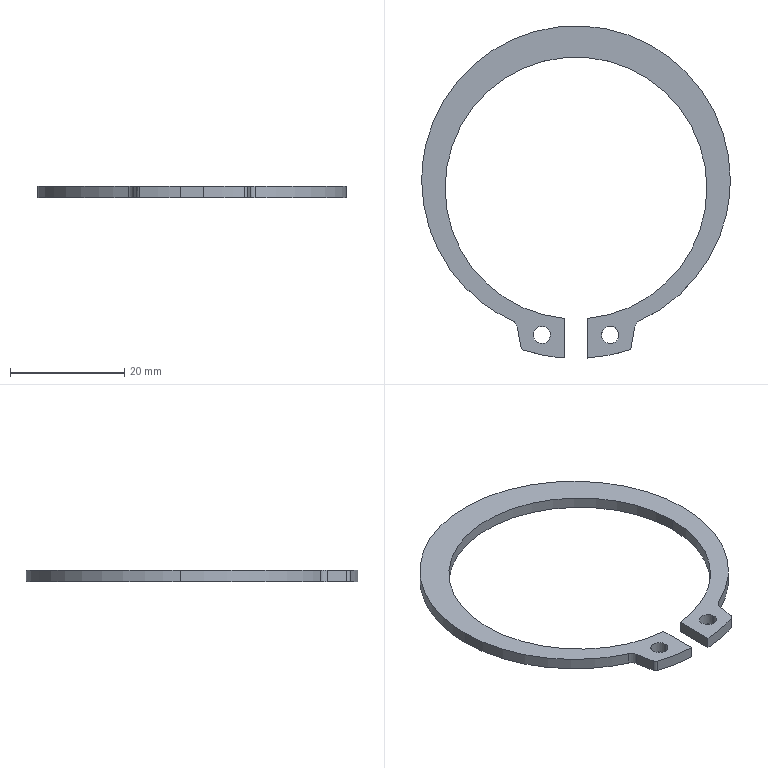Part | STEP file | PN_0041_Default<As Machined> | 1 solid | 22 faces | box 54 x 58.103 x 2 mm | volume 1371 mm3 | cylinder 16 | plane 6 | commonest cylinder face diameters 3 x6 45.8 x3 54 x3 1.4 x2 59.6 x2
STEP:
#1=CARTESIAN_POINT('',(4.5,-27.079,-2.));
#2=VERTEX_POINT('',#1);
#3=CARTESIAN_POINT('',(7.5,-27.079,-2.));
#4=VERTEX_POINT('',#3);
#5=CARTESIAN_POINT('',(6.,-27.079,-2.));
#6=DIRECTION('',(0.,0.,1.));
#7=AXIS2_PLACEMENT_3D('',#5,#6,$);
#8=CIRCLE('',#7,1.5);
#9=EDGE_CURVE('',#2,#4,#8,.T.);
#10=ORIENTED_EDGE('',*,*,#9,.F.);
#11=CARTESIAN_POINT('',(4.5,-27.079,0.));
#12=VERTEX_POINT('',#11);
#13=CARTESIAN_POINT('',(4.5,-27.079,-2.));
#14=DIRECTION('',(0.,0.,1.));
#15=VECTOR('',#14,1.);
#16=LINE('',#13,#15);
#17=EDGE_CURVE('',#2,#12,#16,.T.);
#18=ORIENTED_EDGE('',*,*,#17,.T.);
#19=CARTESIAN_POINT('',(7.5,-27.079,0.));
#20=VERTEX_POINT('',#19);
#21=CARTESIAN_POINT('',(6.,-27.079,0.));
#22=DIRECTION('',(0.,0.,1.));
#23=AXIS2_PLACEMENT_3D('',#21,#22,$);
#24=CIRCLE('',#23,1.5);
#25=EDGE_CURVE('',#12,#20,#24,.T.);
#26=ORIENTED_EDGE('',*,*,#25,.T.);
#27=CARTESIAN_POINT('',(7.5,-27.079,-2.));
#28=DIRECTION('',(0.,0.,1.));
#29=VECTOR('',#28,1.);
#30=LINE('',#27,#29);
#31=EDGE_CURVE('',#4,#20,#30,.T.);
#32=ORIENTED_EDGE('',*,*,#31,.F.);
#33=EDGE_LOOP('',(#10,#18,#26,#32));
#34=FACE_OUTER_BOUND('',#33,.T.);
#35=CARTESIAN_POINT('',(6.,-27.079,-2.));
#36=DIRECTION('',(0.,0.,1.));
#37=DIRECTION('',(-1.,0.,0.));
#38=AXIS2_PLACEMENT_3D('',#35,#36,#37);
#39=CYLINDRICAL_SURFACE('',#38,1.5);
#40=ADVANCED_FACE('',(#34),#39,.F.);
#41=CARTESIAN_POINT('',(-9.187,-29.719,-2.));
#42=VERTEX_POINT('',#41);
#43=CARTESIAN_POINT('',(-2.,-31.103,-2.));
#44=VERTEX_POINT('',#43);
#45=CARTESIAN_POINT('',(-9.187,-29.719,-2.));
#46=CARTESIAN_POINT('',(-7.791,-30.171,-2.));
#47=CARTESIAN_POINT('',(-6.367,-30.537,-2.));
#48=CARTESIAN_POINT('',(-4.922,-30.816,-2.));
#49=CARTESIAN_POINT('',(-3.464,-31.004,-2.));
#50=CARTESIAN_POINT('',(-2.,-31.103,-2.));
#51=B_SPLINE_CURVE_WITH_KNOTS('',5,(#45,#46,#47,#48,#49,#50),.UNSPECIFIED.,.F.,.U.,(6,6),(0.,10.377),.UNSPECIFIED.);
#52=EDGE_CURVE('',#42,#44,#51,.T.);
#53=ORIENTED_EDGE('',*,*,#52,.F.);
#54=CARTESIAN_POINT('',(-9.66,-29.174,-2.));
#55=VERTEX_POINT('',#54);
#56=CARTESIAN_POINT('',(-8.971,-29.053,-2.));
#57=DIRECTION('',(0.,0.,-1.));
#58=AXIS2_PLACEMENT_3D('',#56,#57,$);
#59=CIRCLE('',#58,0.7);
#60=EDGE_CURVE('',#42,#55,#59,.T.);
#61=ORIENTED_EDGE('',*,*,#60,.T.);
#62=CARTESIAN_POINT('',(-10.272,-25.705,-2.));
#63=VERTEX_POINT('',#62);
#64=CARTESIAN_POINT('',(-9.966,-27.44,-2.));
#65=DIRECTION('',(0.1736,-0.9848,0.));
#66=VECTOR('',#65,1.);
#67=LINE('',#64,#66);
#68=EDGE_CURVE('',#63,#55,#67,.T.);
#69=ORIENTED_EDGE('',*,*,#68,.F.);
#70=CARTESIAN_POINT('',(-11.131,-24.599,-2.));
#71=VERTEX_POINT('',#70);
#72=CARTESIAN_POINT('',(-10.272,-25.705,-2.));
#73=CARTESIAN_POINT('',(-10.303,-25.533,-2.));
#74=CARTESIAN_POINT('',(-10.358,-25.365,-2.));
#75=CARTESIAN_POINT('',(-10.438,-25.207,-2.));
#76=CARTESIAN_POINT('',(-10.607,-24.966,-2.));
#77=CARTESIAN_POINT('',(-10.828,-24.773,-2.));
#78=CARTESIAN_POINT('',(-10.923,-24.705,-2.));
#79=CARTESIAN_POINT('',(-11.025,-24.647,-2.));
#80=CARTESIAN_POINT('',(-11.131,-24.599,-2.));
#81=B_SPLINE_CURVE_WITH_KNOTS('',5,(#72,#73,#74,#75,#76,#77,#78,#79,#80),.UNSPECIFIED.,.F.,.U.,(6,3,6),(0.,1.236,2.06),.UNSPECIFIED.);
#82=EDGE_CURVE('',#63,#71,#81,.T.);
#83=ORIENTED_EDGE('',*,*,#82,.T.);
#84=CARTESIAN_POINT('',(-27.,0.,-2.));
#85=VERTEX_POINT('',#84);
#86=CARTESIAN_POINT('',(-27.,-0.000000001,-2.));
#87=CARTESIAN_POINT('',(-27.,-2.546,-2.));
#88=CARTESIAN_POINT('',(-26.7,-5.091,-2.));
#89=CARTESIAN_POINT('',(-26.1,-7.59,-2.));
#90=CARTESIAN_POINT('',(-24.322,-12.398,-2.));
#91=CARTESIAN_POINT('',(-21.476,-16.661,-2.));
#92=CARTESIAN_POINT('',(-19.807,-18.615,-2.));
#93=CARTESIAN_POINT('',(-17.111,-21.102,-2.));
#94=CARTESIAN_POINT('',(-14.056,-23.092,-2.));
#95=CARTESIAN_POINT('',(-13.106,-23.644,-2.));
#96=CARTESIAN_POINT('',(-12.13,-24.147,-2.));
#97=CARTESIAN_POINT('',(-11.131,-24.599,-2.));
#98=B_SPLINE_CURVE_WITH_KNOTS('',5,(#86,#87,#88,#89,#90,#91,#92,#93,#94,#95,#96,#97),.UNSPECIFIED.,.F.,.U.,(6,3,3,6),(0.,18.,36.,43.753),.UNSPECIFIED.);
#99=EDGE_CURVE('',#85,#71,#98,.T.);
#100=ORIENTED_EDGE('',*,*,#99,.F.);
#101=CARTESIAN_POINT('',(27.,0.,-2.));
#102=VERTEX_POINT('',#101);
#103=CARTESIAN_POINT('',(27.,-0.000000001,-2.));
#104=CARTESIAN_POINT('',(27.,2.546,-2.));
#105=CARTESIAN_POINT('',(26.7,5.091,-2.));
#106=CARTESIAN_POINT('',(26.1,7.59,-2.));
#107=CARTESIAN_POINT('',(24.322,12.398,-2.));
#108=CARTESIAN_POINT('',(21.476,16.661,-2.));
#109=CARTESIAN_POINT('',(19.807,18.615,-2.));
#110=CARTESIAN_POINT('',(16.039,22.091,-2.));
#111=CARTESIAN_POINT('',(11.567,24.597,-2.));
#112=CARTESIAN_POINT('',(9.193,25.579,-2.));
#113=CARTESIAN_POINT('',(4.257,26.966,-2.));
#114=CARTESIAN_POINT('',(-0.8651,27.167,-2.));
#115=CARTESIAN_POINT('',(-3.427,26.964,-2.));
#116=CARTESIAN_POINT('',(-8.453,25.958,-2.));
#117=CARTESIAN_POINT('',(-13.108,23.811,-2.));
#118=CARTESIAN_POINT('',(-15.298,22.467,-2.));
#119=CARTESIAN_POINT('',(-19.32,19.288,-2.));
#120=CARTESIAN_POINT('',(-22.492,15.261,-2.));
#121=CARTESIAN_POINT('',(-23.833,13.069,-2.));
#122=CARTESIAN_POINT('',(-25.613,9.192,-2.));
#123=CARTESIAN_POINT('',(-26.603,5.059,-2.));
#124=CARTESIAN_POINT('',(-26.868,3.382,-2.));
#125=CARTESIAN_POINT('',(-27.,1.691,-2.));
#126=CARTESIAN_POINT('',(-27.,-0.000000001,-2.));
#127=B_SPLINE_CURVE_WITH_KNOTS('',5,(#103,#104,#105,#106,#107,#108,#109,#110,#111,#112,#113,#114,#115,#116,#117,#118,#119,#120,#121,#122,#123,#124,#125,#126),.UNSPECIFIED.,.F.,.U.,(6,3,3,3,3,3,3,6),(0.,18.,36.,54.,71.999,89.999,107.999,119.957),.UNSPECIFIED.);
#128=EDGE_CURVE('',#102,#85,#127,.T.);
#129=ORIENTED_EDGE('',*,*,#128,.F.);
#130=CARTESIAN_POINT('',(11.131,-24.599,-2.));
#131=VERTEX_POINT('',#130);
#132=CARTESIAN_POINT('',(11.131,-24.599,-2.));
#133=CARTESIAN_POINT('',(13.45,-23.549,-2.));
#134=CARTESIAN_POINT('',(15.646,-22.227,-2.));
#135=CARTESIAN_POINT('',(17.675,-20.65,-2.));
#136=CARTESIAN_POINT('',(21.323,-17.048,-2.));
#137=CARTESIAN_POINT('',(24.033,-12.697,-2.));
#138=CARTESIAN_POINT('',(25.125,-10.371,-2.));
#139=CARTESIAN_POINT('',(26.28,-6.89,-2.));
#140=CARTESIAN_POINT('',(26.833,-3.286,-2.));
#141=CARTESIAN_POINT('',(26.944,-2.193,-2.));
#142=CARTESIAN_POINT('',(27.,-1.096,-2.));
#143=CARTESIAN_POINT('',(27.,-0.000000001,-2.));
#144=B_SPLINE_CURVE_WITH_KNOTS('',5,(#132,#133,#134,#135,#136,#137,#138,#139,#140,#141,#142,#143),.UNSPECIFIED.,.F.,.U.,(6,3,3,6),(0.,18.,36.,43.753),.UNSPECIFIED.);
#145=EDGE_CURVE('',#131,#102,#144,.T.);
#146=ORIENTED_EDGE('',*,*,#145,.F.);
#147=CARTESIAN_POINT('',(10.272,-25.705,-2.));
#148=VERTEX_POINT('',#147);
#149=CARTESIAN_POINT('',(11.131,-24.599,-2.));
#150=CARTESIAN_POINT('',(10.972,-24.671,-2.));
#151=CARTESIAN_POINT('',(10.823,-24.766,-2.));
#152=CARTESIAN_POINT('',(10.689,-24.883,-2.));
#153=CARTESIAN_POINT('',(10.498,-25.106,-2.));
#154=CARTESIAN_POINT('',(10.366,-25.368,-2.));
#155=CARTESIAN_POINT('',(10.324,-25.477,-2.));
#156=CARTESIAN_POINT('',(10.292,-25.59,-2.));
#157=CARTESIAN_POINT('',(10.272,-25.705,-2.));
#158=B_SPLINE_CURVE_WITH_KNOTS('',5,(#149,#150,#151,#152,#153,#154,#155,#156,#157),.UNSPECIFIED.,.F.,.U.,(6,3,6),(0.,1.236,2.06),.UNSPECIFIED.);
#159=EDGE_CURVE('',#131,#148,#158,.T.);
#160=ORIENTED_EDGE('',*,*,#159,.T.);
#161=CARTESIAN_POINT('',(9.66,-29.174,-2.));
#162=VERTEX_POINT('',#161);
#163=CARTESIAN_POINT('',(9.966,-27.44,-2.));
#164=DIRECTION('',(0.1736,0.9848,0.));
#165=VECTOR('',#164,1.);
#166=LINE('',#163,#165);
#167=EDGE_CURVE('',#162,#148,#166,.T.);
#168=ORIENTED_EDGE('',*,*,#167,.F.);
#169=CARTESIAN_POINT('',(9.187,-29.719,-2.));
#170=VERTEX_POINT('',#169);
#171=CARTESIAN_POINT('',(8.971,-29.053,-2.));
#172=DIRECTION('',(0.,0.,-1.));
#173=AXIS2_PLACEMENT_3D('',#171,#172,$);
#174=CIRCLE('',#173,0.7);
#175=EDGE_CURVE('',#162,#170,#174,.T.);
#176=ORIENTED_EDGE('',*,*,#175,.T.);
#177=CARTESIAN_POINT('',(2.,-31.103,-2.));
#178=VERTEX_POINT('',#177);
#179=CARTESIAN_POINT('',(2.,-31.103,-2.));
#180=CARTESIAN_POINT('',(3.464,-31.004,-2.));
#181=CARTESIAN_POINT('',(4.922,-30.816,-2.));
#182=CARTESIAN_POINT('',(6.367,-30.537,-2.));
#183=CARTESIAN_POINT('',(7.791,-30.171,-2.));
#184=CARTESIAN_POINT('',(9.187,-29.719,-2.));
#185=B_SPLINE_CURVE_WITH_KNOTS('',5,(#179,#180,#181,#182,#183,#184),.UNSPECIFIED.,.F.,.U.,(6,6),(0.,10.377),.UNSPECIFIED.);
#186=EDGE_CURVE('',#178,#170,#185,.T.);
#187=ORIENTED_EDGE('',*,*,#186,.F.);
#188=CARTESIAN_POINT('',(2.,-24.182,-2.));
#189=VERTEX_POINT('',#188);
#190=CARTESIAN_POINT('',(2.,-27.643,-2.));
#191=DIRECTION('',(0.,-1.,0.));
#192=VECTOR('',#191,1.);
#193=LINE('',#190,#192);
#194=EDGE_CURVE('',#189,#178,#193,.T.);
#195=ORIENTED_EDGE('',*,*,#194,.F.);
#196=CARTESIAN_POINT('',(22.9,-1.37,-2.));
#197=VERTEX_POINT('',#196);
#198=CARTESIAN_POINT('',(0.000000001,-1.37,-2.));
#199=DIRECTION('',(0.,0.,-1.));
#200=AXIS2_PLACEMENT_3D('',#198,#199,$);
#201=CIRCLE('',#200,22.9);
#202=EDGE_CURVE('',#197,#189,#201,.T.);
#203=ORIENTED_EDGE('',*,*,#202,.F.);
#204=CARTESIAN_POINT('',(-22.9,-1.37,-2.));
#205=VERTEX_POINT('',#204);
#206=CARTESIAN_POINT('',(0.,-1.37,-2.));
#207=DIRECTION('',(0.,0.,-1.));
#208=AXIS2_PLACEMENT_3D('',#206,#207,$);
#209=CIRCLE('',#208,22.9);
#210=EDGE_CURVE('',#205,#197,#209,.T.);
#211=ORIENTED_EDGE('',*,*,#210,.F.);
#212=CARTESIAN_POINT('',(-2.,-24.182,-2.));
#213=VERTEX_POINT('',#212);
#214=CARTESIAN_POINT('',(-0.000000001,-1.37,-2.));
#215=DIRECTION('',(0.,0.,-1.));
#216=AXIS2_PLACEMENT_3D('',#214,#215,$);
#217=CIRCLE('',#216,22.9);
#218=EDGE_CURVE('',#213,#205,#217,.T.);
#219=ORIENTED_EDGE('',*,*,#218,.F.);
#220=CARTESIAN_POINT('',(-2.,-27.643,-2.));
#221=DIRECTION('',(0.,1.,0.));
#222=VECTOR('',#221,1.);
#223=LINE('',#220,#222);
#224=EDGE_CURVE('',#44,#213,#223,.T.);
#225=ORIENTED_EDGE('',*,*,#224,.F.);
#226=EDGE_LOOP('',(#53,#61,#69,#83,#100,#129,#146,#160,#168,#176,#187,#195,#203,#211,#219,#225));
#227=FACE_OUTER_BOUND('',#226,.T.);
#228=CARTESIAN_POINT('',(7.5,-27.079,-2.));
#229=CARTESIAN_POINT('',(7.5,-26.899,-2.));
#230=CARTESIAN_POINT('',(7.473,-26.719,-2.));
#231=CARTESIAN_POINT('',(7.419,-26.545,-2.));
#232=CARTESIAN_POINT('',(7.26,-26.217,-2.));
#233=CARTESIAN_POINT('',(7.012,-25.95,-2.));
#234=CARTESIAN_POINT('',(6.869,-25.837,-2.));
#235=CARTESIAN_POINT('',(6.553,-25.656,-2.));
#236=CARTESIAN_POINT('',(6.198,-25.576,-2.));
#237=CARTESIAN_POINT('',(6.016,-25.563,-2.));
#238=CARTESIAN_POINT('',(5.653,-25.592,-2.));
#239=CARTESIAN_POINT('',(5.315,-25.726,-2.));
#240=CARTESIAN_POINT('',(5.157,-25.819,-2.));
#241=CARTESIAN_POINT('',(4.874,-26.048,-2.));
#242=CARTESIAN_POINT('',(4.671,-26.35,-2.));
#243=CARTESIAN_POINT('',(4.593,-26.515,-2.));
#244=CARTESIAN_POINT('',(4.528,-26.73,-2.));
#245=CARTESIAN_POINT('',(4.505,-26.952,-2.));
#246=CARTESIAN_POINT('',(4.502,-26.994,-2.));
#247=CARTESIAN_POINT('',(4.5,-27.037,-2.));
#248=CARTESIAN_POINT('',(4.5,-27.079,-2.));
#249=B_SPLINE_CURVE_WITH_KNOTS('',5,(#228,#229,#230,#231,#232,#233,#234,#235,#236,#237,#238,#239,#240,#241,#242,#243,#244,#245,#246,#247,#248),.UNSPECIFIED.,.F.,.U.,(6,3,3,3,3,3,6),(0.,1.273,2.546,3.818,5.091,6.364,6.664),.UNSPECIFIED.);
#250=EDGE_CURVE('',#4,#2,#249,.T.);
#251=ORIENTED_EDGE('',*,*,#250,.T.);
#252=ORIENTED_EDGE('',*,*,#9,.T.);
#253=EDGE_LOOP('',(#251,#252));
#254=FACE_BOUND('',#253,.T.);
#255=CARTESIAN_POINT('',(-4.5,-27.079,-2.));
#256=VERTEX_POINT('',#255);
#257=CARTESIAN_POINT('',(-7.5,-27.079,-2.));
#258=VERTEX_POINT('',#257);
#259=CARTESIAN_POINT('',(-4.5,-27.079,-2.));
#260=CARTESIAN_POINT('',(-4.5,-26.899,-2.));
#261=CARTESIAN_POINT('',(-4.527,-26.719,-2.));
#262=CARTESIAN_POINT('',(-4.581,-26.545,-2.));
#263=CARTESIAN_POINT('',(-4.74,-26.217,-2.));
#264=CARTESIAN_POINT('',(-4.988,-25.95,-2.));
#265=CARTESIAN_POINT('',(-5.131,-25.837,-2.));
#266=CARTESIAN_POINT('',(-5.447,-25.656,-2.));
#267=CARTESIAN_POINT('',(-5.802,-25.576,-2.));
#268=CARTESIAN_POINT('',(-5.984,-25.563,-2.));
#269=CARTESIAN_POINT('',(-6.347,-25.592,-2.));
#270=CARTESIAN_POINT('',(-6.685,-25.726,-2.));
#271=CARTESIAN_POINT('',(-6.843,-25.819,-2.));
#272=CARTESIAN_POINT('',(-7.126,-26.048,-2.));
#273=CARTESIAN_POINT('',(-7.329,-26.35,-2.));
#274=CARTESIAN_POINT('',(-7.407,-26.515,-2.));
#275=CARTESIAN_POINT('',(-7.472,-26.73,-2.));
#276=CARTESIAN_POINT('',(-7.495,-26.952,-2.));
#277=CARTESIAN_POINT('',(-7.498,-26.994,-2.));
#278=CARTESIAN_POINT('',(-7.5,-27.037,-2.));
#279=CARTESIAN_POINT('',(-7.5,-27.079,-2.));
#280=B_SPLINE_CURVE_WITH_KNOTS('',5,(#259,#260,#261,#262,#263,#264,#265,#266,#267,#268,#269,#270,#271,#272,#273,#274,#275,#276,#277,#278,#279),.UNSPECIFIED.,.F.,.U.,(6,3,3,3,3,3,6),(0.,1.273,2.546,3.818,5.091,6.364,6.664),.UNSPECIFIED.);
#281=EDGE_CURVE('',#256,#258,#280,.T.);
#282=ORIENTED_EDGE('',*,*,#281,.T.);
#283=CARTESIAN_POINT('',(-7.5,-27.079,-2.));
#284=CARTESIAN_POINT('',(-7.5,-27.259,-2.));
#285=CARTESIAN_POINT('',(-7.473,-27.439,-2.));
#286=CARTESIAN_POINT('',(-7.419,-27.614,-2.));
#287=CARTESIAN_POINT('',(-7.26,-27.941,-2.));
#288=CARTESIAN_POINT('',(-7.012,-28.208,-2.));
#289=CARTESIAN_POINT('',(-6.869,-28.322,-2.));
#290=CARTESIAN_POINT('',(-6.553,-28.502,-2.));
#291=CARTESIAN_POINT('',(-6.198,-28.582,-2.));
#292=CARTESIAN_POINT('',(-6.016,-28.595,-2.));
#293=CARTESIAN_POINT('',(-5.653,-28.566,-2.));
#294=CARTESIAN_POINT('',(-5.315,-28.432,-2.));
#295=CARTESIAN_POINT('',(-5.157,-28.34,-2.));
#296=CARTESIAN_POINT('',(-4.874,-28.111,-2.));
#297=CARTESIAN_POINT('',(-4.671,-27.809,-2.));
#298=CARTESIAN_POINT('',(-4.593,-27.643,-2.));
#299=CARTESIAN_POINT('',(-4.528,-27.428,-2.));
#300=CARTESIAN_POINT('',(-4.505,-27.207,-2.));
#301=CARTESIAN_POINT('',(-4.502,-27.164,-2.));
#302=CARTESIAN_POINT('',(-4.5,-27.122,-2.));
#303=CARTESIAN_POINT('',(-4.5,-27.079,-2.));
#304=B_SPLINE_CURVE_WITH_KNOTS('',5,(#283,#284,#285,#286,#287,#288,#289,#290,#291,#292,#293,#294,#295,#296,#297,#298,#299,#300,#301,#302,#303),.UNSPECIFIED.,.F.,.U.,(6,3,3,3,3,3,6),(0.,1.273,2.546,3.818,5.091,6.364,6.664),.UNSPECIFIED.);
#305=EDGE_CURVE('',#258,#256,#304,.T.);
#306=ORIENTED_EDGE('',*,*,#305,.T.);
#307=EDGE_LOOP('',(#282,#306));
#308=FACE_BOUND('',#307,.T.);
#309=CARTESIAN_POINT('',(0.,-1.37,-2.));
#310=DIRECTION('',(0.,0.,-1.));
#311=DIRECTION('',(-1.,0.,0.));
#312=AXIS2_PLACEMENT_3D('',#309,#310,#311);
#313=PLANE('',#312);
#314=ADVANCED_FACE('',(#227,#254,#308),#313,.T.);
#315=ORIENTED_EDGE('',*,*,#17,.F.);
#316=ORIENTED_EDGE('',*,*,#250,.F.);
#317=ORIENTED_EDGE('',*,*,#31,.T.);
#318=CARTESIAN_POINT('',(6.,-27.079,0.));
#319=DIRECTION('',(0.,0.,1.));
#320=AXIS2_PLACEMENT_3D('',#318,#319,$);
#321=CIRCLE('',#320,1.5);
#322=EDGE_CURVE('',#20,#12,#321,.T.);
#323=ORIENTED_EDGE('',*,*,#322,.T.);
#324=EDGE_LOOP('',(#315,#316,#317,#323));
#325=FACE_OUTER_BOUND('',#324,.T.);
#326=CARTESIAN_POINT('',(6.,-27.079,-2.));
#327=DIRECTION('',(0.,0.,1.));
#328=DIRECTION('',(1.,0.,0.));
#329=AXIS2_PLACEMENT_3D('',#326,#327,#328);
#330=CYLINDRICAL_SURFACE('',#329,1.5);
#331=ADVANCED_FACE('',(#325),#330,.F.);
#332=CARTESIAN_POINT('',(11.131,-24.599,0.));
#333=VERTEX_POINT('',#332);
#334=CARTESIAN_POINT('',(27.,0.,0.));
#335=VERTEX_POINT('',#334);
#336=CARTESIAN_POINT('',(11.131,-24.599,0.));
#337=CARTESIAN_POINT('',(13.45,-23.549,0.));
#338=CARTESIAN_POINT('',(15.646,-22.227,0.));
#339=CARTESIAN_POINT('',(17.675,-20.65,0.));
#340=CARTESIAN_POINT('',(21.323,-17.048,0.));
#341=CARTESIAN_POINT('',(24.033,-12.697,0.));
#342=CARTESIAN_POINT('',(25.125,-10.371,0.));
#343=CARTESIAN_POINT('',(26.28,-6.89,0.));
#344=CARTESIAN_POINT('',(26.833,-3.286,0.));
#345=CARTESIAN_POINT('',(26.944,-2.193,0.));
#346=CARTESIAN_POINT('',(27.,-1.096,0.));
#347=CARTESIAN_POINT('',(27.,-0.000000001,0.));
#348=B_SPLINE_CURVE_WITH_KNOTS('',5,(#336,#337,#338,#339,#340,#341,#342,#343,#344,#345,#346,#347),.UNSPECIFIED.,.F.,.U.,(6,3,3,6),(0.,18.,36.,43.753),.UNSPECIFIED.);
#349=EDGE_CURVE('',#333,#335,#348,.T.);
#350=ORIENTED_EDGE('',*,*,#349,.T.);
#351=CARTESIAN_POINT('',(-27.,0.,0.));
#352=VERTEX_POINT('',#351);
#353=CARTESIAN_POINT('',(27.,-0.000000001,0.));
#354=CARTESIAN_POINT('',(27.,2.546,0.));
#355=CARTESIAN_POINT('',(26.7,5.091,0.));
#356=CARTESIAN_POINT('',(26.1,7.59,0.));
#357=CARTESIAN_POINT('',(24.322,12.398,0.));
#358=CARTESIAN_POINT('',(21.476,16.661,0.));
#359=CARTESIAN_POINT('',(19.807,18.615,0.));
#360=CARTESIAN_POINT('',(16.039,22.091,0.));
#361=CARTESIAN_POINT('',(11.567,24.597,0.));
#362=CARTESIAN_POINT('',(9.193,25.579,0.));
#363=CARTESIAN_POINT('',(4.257,26.966,0.));
#364=CARTESIAN_POINT('',(-0.8651,27.167,0.));
#365=CARTESIAN_POINT('',(-3.427,26.964,0.));
#366=CARTESIAN_POINT('',(-8.453,25.958,0.));
#367=CARTESIAN_POINT('',(-13.108,23.811,0.));
#368=CARTESIAN_POINT('',(-15.298,22.467,0.));
#369=CARTESIAN_POINT('',(-19.32,19.288,0.));
#370=CARTESIAN_POINT('',(-22.492,15.261,0.));
#371=CARTESIAN_POINT('',(-23.833,13.069,0.));
#372=CARTESIAN_POINT('',(-25.613,9.192,0.));
#373=CARTESIAN_POINT('',(-26.603,5.059,0.));
#374=CARTESIAN_POINT('',(-26.868,3.382,0.));
#375=CARTESIAN_POINT('',(-27.,1.691,0.));
#376=CARTESIAN_POINT('',(-27.,-0.000000001,0.));
#377=B_SPLINE_CURVE_WITH_KNOTS('',5,(#353,#354,#355,#356,#357,#358,#359,#360,#361,#362,#363,#364,#365,#366,#367,#368,#369,#370,#371,#372,#373,#374,#375,#376),.UNSPECIFIED.,.F.,.U.,(6,3,3,3,3,3,3,6),(0.,18.,36.,54.,71.999,89.999,107.999,119.957),.UNSPECIFIED.);
#378=EDGE_CURVE('',#335,#352,#377,.T.);
#379=ORIENTED_EDGE('',*,*,#378,.T.);
#380=CARTESIAN_POINT('',(-11.131,-24.599,0.));
#381=VERTEX_POINT('',#380);
#382=CARTESIAN_POINT('',(-27.,-0.000000001,0.));
#383=CARTESIAN_POINT('',(-27.,-2.546,0.));
#384=CARTESIAN_POINT('',(-26.7,-5.091,0.));
#385=CARTESIAN_POINT('',(-26.1,-7.59,0.));
#386=CARTESIAN_POINT('',(-24.322,-12.398,0.));
#387=CARTESIAN_POINT('',(-21.476,-16.661,0.));
#388=CARTESIAN_POINT('',(-19.807,-18.615,0.));
#389=CARTESIAN_POINT('',(-17.111,-21.102,0.));
#390=CARTESIAN_POINT('',(-14.056,-23.092,0.));
#391=CARTESIAN_POINT('',(-13.106,-23.644,0.));
#392=CARTESIAN_POINT('',(-12.13,-24.147,0.));
#393=CARTESIAN_POINT('',(-11.131,-24.599,0.));
#394=B_SPLINE_CURVE_WITH_KNOTS('',5,(#382,#383,#384,#385,#386,#387,#388,#389,#390,#391,#392,#393),.UNSPECIFIED.,.F.,.U.,(6,3,3,6),(0.,18.,36.,43.753),.UNSPECIFIED.);
#395=EDGE_CURVE('',#352,#381,#394,.T.);
#396=ORIENTED_EDGE('',*,*,#395,.T.);
#397=CARTESIAN_POINT('',(-10.272,-25.705,0.));
#398=VERTEX_POINT('',#397);
#399=CARTESIAN_POINT('',(-11.749,-25.965,0.));
#400=DIRECTION('',(0.,0.,-1.));
#401=AXIS2_PLACEMENT_3D('',#399,#400,$);
#402=CIRCLE('',#401,1.5);
#403=EDGE_CURVE('',#381,#398,#402,.T.);
#404=ORIENTED_EDGE('',*,*,#403,.T.);
#405=CARTESIAN_POINT('',(-9.66,-29.174,0.));
#406=VERTEX_POINT('',#405);
#407=CARTESIAN_POINT('',(-9.966,-27.44,0.));
#408=DIRECTION('',(0.1736,-0.9848,0.));
#409=VECTOR('',#408,1.);
#410=LINE('',#407,#409);
#411=EDGE_CURVE('',#398,#406,#410,.T.);
#412=ORIENTED_EDGE('',*,*,#411,.T.);
#413=CARTESIAN_POINT('',(-9.187,-29.719,0.));
#414=VERTEX_POINT('',#413);
#415=CARTESIAN_POINT('',(-9.66,-29.174,0.));
#416=CARTESIAN_POINT('',(-9.645,-29.264,0.));
#417=CARTESIAN_POINT('',(-9.614,-29.351,0.));
#418=CARTESIAN_POINT('',(-9.57,-29.432,0.));
#419=CARTESIAN_POINT('',(-9.475,-29.553,0.));
#420=CARTESIAN_POINT('',(-9.353,-29.644,0.));
#421=CARTESIAN_POINT('',(-9.3,-29.675,0.));
#422=CARTESIAN_POINT('',(-9.245,-29.7,0.));
#423=CARTESIAN_POINT('',(-9.187,-29.719,0.));
#424=B_SPLINE_CURVE_WITH_KNOTS('',5,(#415,#416,#417,#418,#419,#420,#421,#422,#423),.UNSPECIFIED.,.F.,.U.,(6,3,6),(0.,0.6432,1.072),.UNSPECIFIED.);
#425=EDGE_CURVE('',#406,#414,#424,.T.);
#426=ORIENTED_EDGE('',*,*,#425,.T.);
#427=CARTESIAN_POINT('',(-2.,-31.103,0.));
#428=VERTEX_POINT('',#427);
#429=CARTESIAN_POINT('',(-9.187,-29.719,0.));
#430=CARTESIAN_POINT('',(-7.791,-30.171,0.));
#431=CARTESIAN_POINT('',(-6.367,-30.537,0.));
#432=CARTESIAN_POINT('',(-4.922,-30.816,0.));
#433=CARTESIAN_POINT('',(-3.464,-31.004,0.));
#434=CARTESIAN_POINT('',(-2.,-31.103,0.));
#435=B_SPLINE_CURVE_WITH_KNOTS('',5,(#429,#430,#431,#432,#433,#434),.UNSPECIFIED.,.F.,.U.,(6,6),(0.,10.377),.UNSPECIFIED.);
#436=EDGE_CURVE('',#414,#428,#435,.T.);
#437=ORIENTED_EDGE('',*,*,#436,.T.);
#438=CARTESIAN_POINT('',(-2.,-24.182,0.));
#439=VERTEX_POINT('',#438);
#440=CARTESIAN_POINT('',(-2.,-27.643,0.));
#441=DIRECTION('',(0.,1.,0.));
#442=VECTOR('',#441,1.);
#443=LINE('',#440,#442);
#444=EDGE_CURVE('',#428,#439,#443,.T.);
#445=ORIENTED_EDGE('',*,*,#444,.T.);
#446=CARTESIAN_POINT('',(-22.9,-1.37,0.));
#447=VERTEX_POINT('',#446);
#448=CARTESIAN_POINT('',(-0.000000001,-1.37,0.));
#449=DIRECTION('',(0.,0.,-1.));
#450=AXIS2_PLACEMENT_3D('',#448,#449,$);
#451=CIRCLE('',#450,22.9);
#452=EDGE_CURVE('',#439,#447,#451,.T.);
#453=ORIENTED_EDGE('',*,*,#452,.T.);
#454=CARTESIAN_POINT('',(22.9,-1.37,0.));
#455=VERTEX_POINT('',#454);
#456=CARTESIAN_POINT('',(0.,-1.37,0.));
#457=DIRECTION('',(0.,0.,-1.));
#458=AXIS2_PLACEMENT_3D('',#456,#457,$);
#459=CIRCLE('',#458,22.9);
#460=EDGE_CURVE('',#447,#455,#459,.T.);
#461=ORIENTED_EDGE('',*,*,#460,.T.);
#462=CARTESIAN_POINT('',(2.,-24.182,0.));
#463=VERTEX_POINT('',#462);
#464=CARTESIAN_POINT('',(0.000000001,-1.37,0.));
#465=DIRECTION('',(0.,0.,-1.));
#466=AXIS2_PLACEMENT_3D('',#464,#465,$);
#467=CIRCLE('',#466,22.9);
#468=EDGE_CURVE('',#455,#463,#467,.T.);
#469=ORIENTED_EDGE('',*,*,#468,.T.);
#470=CARTESIAN_POINT('',(2.,-31.103,0.));
#471=VERTEX_POINT('',#470);
#472=CARTESIAN_POINT('',(2.,-27.643,0.));
#473=DIRECTION('',(0.,-1.,0.));
#474=VECTOR('',#473,1.);
#475=LINE('',#472,#474);
#476=EDGE_CURVE('',#463,#471,#475,.T.);
#477=ORIENTED_EDGE('',*,*,#476,.T.);
#478=CARTESIAN_POINT('',(9.187,-29.719,0.));
#479=VERTEX_POINT('',#478);
#480=CARTESIAN_POINT('',(2.,-31.103,0.));
#481=CARTESIAN_POINT('',(3.464,-31.004,0.));
#482=CARTESIAN_POINT('',(4.922,-30.816,0.));
#483=CARTESIAN_POINT('',(6.367,-30.537,0.));
#484=CARTESIAN_POINT('',(7.791,-30.171,0.));
#485=CARTESIAN_POINT('',(9.187,-29.719,0.));
#486=B_SPLINE_CURVE_WITH_KNOTS('',5,(#480,#481,#482,#483,#484,#485),.UNSPECIFIED.,.F.,.U.,(6,6),(0.,10.377),.UNSPECIFIED.);
#487=EDGE_CURVE('',#471,#479,#486,.T.);
#488=ORIENTED_EDGE('',*,*,#487,.T.);
#489=CARTESIAN_POINT('',(9.66,-29.174,0.));
#490=VERTEX_POINT('',#489);
#491=CARTESIAN_POINT('',(9.187,-29.719,0.));
#492=CARTESIAN_POINT('',(9.273,-29.691,0.));
#493=CARTESIAN_POINT('',(9.355,-29.648,0.));
#494=CARTESIAN_POINT('',(9.43,-29.593,0.));
#495=CARTESIAN_POINT('',(9.537,-29.483,0.));
#496=CARTESIAN_POINT('',(9.61,-29.349,0.));
#497=CARTESIAN_POINT('',(9.633,-29.293,0.));
#498=CARTESIAN_POINT('',(9.65,-29.234,0.));
#499=CARTESIAN_POINT('',(9.66,-29.174,0.));
#500=B_SPLINE_CURVE_WITH_KNOTS('',5,(#491,#492,#493,#494,#495,#496,#497,#498,#499),.UNSPECIFIED.,.F.,.U.,(6,3,6),(0.,0.6432,1.072),.UNSPECIFIED.);
#501=EDGE_CURVE('',#479,#490,#500,.T.);
#502=ORIENTED_EDGE('',*,*,#501,.T.);
#503=CARTESIAN_POINT('',(10.272,-25.705,0.));
#504=VERTEX_POINT('',#503);
#505=CARTESIAN_POINT('',(9.966,-27.44,0.));
#506=DIRECTION('',(0.1736,0.9848,0.));
#507=VECTOR('',#506,1.);
#508=LINE('',#505,#507);
#509=EDGE_CURVE('',#490,#504,#508,.T.);
#510=ORIENTED_EDGE('',*,*,#509,.T.);
#511=CARTESIAN_POINT('',(11.749,-25.965,0.));
#512=DIRECTION('',(0.,0.,-1.));
#513=AXIS2_PLACEMENT_3D('',#511,#512,$);
#514=CIRCLE('',#513,1.5);
#515=EDGE_CURVE('',#504,#333,#514,.T.);
#516=ORIENTED_EDGE('',*,*,#515,.T.);
#517=EDGE_LOOP('',(#350,#379,#396,#404,#412,#426,#437,#445,#453,#461,#469,#477,#488,#502,#510,#516));
#518=FACE_OUTER_BOUND('',#517,.T.);
#519=ORIENTED_EDGE('',*,*,#322,.F.);
#520=ORIENTED_EDGE('',*,*,#25,.F.);
#521=EDGE_LOOP('',(#519,#520));
#522=FACE_BOUND('',#521,.T.);
#523=CARTESIAN_POINT('',(-4.5,-27.079,0.));
#524=VERTEX_POINT('',#523);
#525=CARTESIAN_POINT('',(-7.5,-27.079,0.));
#526=VERTEX_POINT('',#525);
#527=CARTESIAN_POINT('',(-4.5,-27.079,0.));
#528=CARTESIAN_POINT('',(-4.5,-26.899,0.));
#529=CARTESIAN_POINT('',(-4.527,-26.719,0.));
#530=CARTESIAN_POINT('',(-4.581,-26.545,0.));
#531=CARTESIAN_POINT('',(-4.74,-26.217,0.));
#532=CARTESIAN_POINT('',(-4.988,-25.95,0.));
#533=CARTESIAN_POINT('',(-5.131,-25.837,0.));
#534=CARTESIAN_POINT('',(-5.447,-25.656,0.));
#535=CARTESIAN_POINT('',(-5.802,-25.576,0.));
#536=CARTESIAN_POINT('',(-5.984,-25.563,0.));
#537=CARTESIAN_POINT('',(-6.347,-25.592,0.));
#538=CARTESIAN_POINT('',(-6.685,-25.726,0.));
#539=CARTESIAN_POINT('',(-6.843,-25.819,0.));
#540=CARTESIAN_POINT('',(-7.126,-26.048,0.));
#541=CARTESIAN_POINT('',(-7.329,-26.35,0.));
#542=CARTESIAN_POINT('',(-7.407,-26.515,0.));
#543=CARTESIAN_POINT('',(-7.472,-26.73,0.));
#544=CARTESIAN_POINT('',(-7.495,-26.952,0.));
#545=CARTESIAN_POINT('',(-7.498,-26.994,0.));
#546=CARTESIAN_POINT('',(-7.5,-27.037,0.));
#547=CARTESIAN_POINT('',(-7.5,-27.079,0.));
#548=B_SPLINE_CURVE_WITH_KNOTS('',5,(#527,#528,#529,#530,#531,#532,#533,#534,#535,#536,#537,#538,#539,#540,#541,#542,#543,#544,#545,#546,#547),.UNSPECIFIED.,.F.,.U.,(6,3,3,3,3,3,6),(0.,1.273,2.546,3.818,5.091,6.364,6.664),.UNSPECIFIED.);
#549=EDGE_CURVE('',#524,#526,#548,.T.);
#550=ORIENTED_EDGE('',*,*,#549,.F.);
#551=CARTESIAN_POINT('',(-7.5,-27.079,0.));
#552=CARTESIAN_POINT('',(-7.5,-27.259,0.));
#553=CARTESIAN_POINT('',(-7.473,-27.439,0.));
#554=CARTESIAN_POINT('',(-7.419,-27.614,0.));
#555=CARTESIAN_POINT('',(-7.26,-27.941,0.));
#556=CARTESIAN_POINT('',(-7.012,-28.208,0.));
#557=CARTESIAN_POINT('',(-6.869,-28.322,0.));
#558=CARTESIAN_POINT('',(-6.553,-28.502,0.));
#559=CARTESIAN_POINT('',(-6.198,-28.582,0.));
#560=CARTESIAN_POINT('',(-6.016,-28.595,0.));
#561=CARTESIAN_POINT('',(-5.653,-28.566,0.));
#562=CARTESIAN_POINT('',(-5.315,-28.432,0.));
#563=CARTESIAN_POINT('',(-5.157,-28.34,0.));
#564=CARTESIAN_POINT('',(-4.874,-28.111,0.));
#565=CARTESIAN_POINT('',(-4.671,-27.809,0.));
#566=CARTESIAN_POINT('',(-4.593,-27.643,0.));
#567=CARTESIAN_POINT('',(-4.528,-27.428,0.));
#568=CARTESIAN_POINT('',(-4.505,-27.207,0.));
#569=CARTESIAN_POINT('',(-4.502,-27.164,0.));
#570=CARTESIAN_POINT('',(-4.5,-27.122,0.));
#571=CARTESIAN_POINT('',(-4.5,-27.079,0.));
#572=B_SPLINE_CURVE_WITH_KNOTS('',5,(#551,#552,#553,#554,#555,#556,#557,#558,#559,#560,#561,#562,#563,#564,#565,#566,#567,#568,#569,#570,#571),.UNSPECIFIED.,.F.,.U.,(6,3,3,3,3,3,6),(0.,1.273,2.546,3.818,5.091,6.364,6.664),.UNSPECIFIED.);
#573=EDGE_CURVE('',#526,#524,#572,.T.);
#574=ORIENTED_EDGE('',*,*,#573,.F.);
#575=EDGE_LOOP('',(#550,#574));
#576=FACE_BOUND('',#575,.T.);
#577=CARTESIAN_POINT('',(0.,-1.37,0.));
#578=DIRECTION('',(0.,0.,-1.));
#579=DIRECTION('',(-1.,0.,0.));
#580=AXIS2_PLACEMENT_3D('',#577,#578,#579);
#581=PLANE('',#580);
#582=ADVANCED_FACE('',(#518,#522,#576),#581,.F.);
#583=ORIENTED_EDGE('',*,*,#436,.F.);
#584=CARTESIAN_POINT('',(-9.187,-29.719,-2.));
#585=DIRECTION('',(0.,0.,1.));
#586=VECTOR('',#585,1.);
#587=LINE('',#584,#586);
#588=EDGE_CURVE('',#414,#42,#587,.F.);
#589=ORIENTED_EDGE('',*,*,#588,.T.);
#590=ORIENTED_EDGE('',*,*,#52,.T.);
#591=CARTESIAN_POINT('',(-2.,-31.103,-2.));
#592=DIRECTION('',(0.,0.,1.));
#593=VECTOR('',#592,1.);
#594=LINE('',#591,#593);
#595=EDGE_CURVE('',#44,#428,#594,.T.);
#596=ORIENTED_EDGE('',*,*,#595,.T.);
#597=EDGE_LOOP('',(#583,#589,#590,#596));
#598=FACE_OUTER_BOUND('',#597,.T.);
#599=CARTESIAN_POINT('',(0.,-1.37,-2.));
#600=DIRECTION('',(0.,0.,1.));
#601=DIRECTION('',(-1.,0.,0.));
#602=AXIS2_PLACEMENT_3D('',#599,#600,#601);
#603=CYLINDRICAL_SURFACE('',#602,29.8);
#604=ADVANCED_FACE('',(#598),#603,.T.);
#605=ORIENTED_EDGE('',*,*,#60,.F.);
#606=ORIENTED_EDGE('',*,*,#588,.F.);
#607=ORIENTED_EDGE('',*,*,#425,.F.);
#608=CARTESIAN_POINT('',(-9.66,-29.174,-2.));
#609=DIRECTION('',(0.,0.,1.));
#610=VECTOR('',#609,1.);
#611=LINE('',#608,#610);
#612=EDGE_CURVE('',#55,#406,#611,.T.);
#613=ORIENTED_EDGE('',*,*,#612,.F.);
#614=EDGE_LOOP('',(#605,#606,#607,#613));
#615=FACE_OUTER_BOUND('',#614,.T.);
#616=CARTESIAN_POINT('',(-8.971,-29.053,-2.));
#617=DIRECTION('',(0.,0.,1.));
#618=DIRECTION('',(-1.,0.,0.));
#619=AXIS2_PLACEMENT_3D('',#616,#617,#618);
#620=CYLINDRICAL_SURFACE('',#619,0.7);
#621=ADVANCED_FACE('',(#615),#620,.T.);
#622=ORIENTED_EDGE('',*,*,#411,.F.);
#623=CARTESIAN_POINT('',(-10.272,-25.705,-1.));
#624=DIRECTION('',(0.,0.,-1.));
#625=VECTOR('',#624,1.);
#626=LINE('',#623,#625);
#627=EDGE_CURVE('',#398,#63,#626,.T.);
#628=ORIENTED_EDGE('',*,*,#627,.T.);
#629=ORIENTED_EDGE('',*,*,#68,.T.);
#630=ORIENTED_EDGE('',*,*,#612,.T.);
#631=EDGE_LOOP('',(#622,#628,#629,#630));
#632=FACE_OUTER_BOUND('',#631,.T.);
#633=CARTESIAN_POINT('',(-10.412,-24.912,-2.));
#634=DIRECTION('',(-0.9848,-0.1736,0.));
#635=DIRECTION('',(0.1736,-0.9848,0.));
#636=AXIS2_PLACEMENT_3D('',#633,#634,#635);
#637=PLANE('',#636);
#638=ADVANCED_FACE('',(#632),#637,.T.);
#639=ORIENTED_EDGE('',*,*,#82,.F.);
#640=ORIENTED_EDGE('',*,*,#627,.F.);
#641=ORIENTED_EDGE('',*,*,#403,.F.);
#642=CARTESIAN_POINT('',(-11.131,-24.599,-2.));
#643=DIRECTION('',(0.,0.,1.));
#644=VECTOR('',#643,1.);
#645=LINE('',#642,#644);
#646=EDGE_CURVE('',#71,#381,#645,.T.);
#647=ORIENTED_EDGE('',*,*,#646,.F.);
#648=EDGE_LOOP('',(#639,#640,#641,#647));
#649=FACE_OUTER_BOUND('',#648,.T.);
#650=CARTESIAN_POINT('',(-11.749,-25.965,-2.));
#651=DIRECTION('',(0.,0.,1.));
#652=DIRECTION('',(1.,0.,0.));
#653=AXIS2_PLACEMENT_3D('',#650,#651,#652);
#654=CYLINDRICAL_SURFACE('',#653,1.5);
#655=ADVANCED_FACE('',(#649),#654,.F.);
#656=CARTESIAN_POINT('',(-27.,0.,-2.));
#657=DIRECTION('',(0.,0.,1.));
#658=VECTOR('',#657,1.);
#659=LINE('',#656,#658);
#660=EDGE_CURVE('',#85,#352,#659,.T.);
#661=ORIENTED_EDGE('',*,*,#660,.F.);
#662=ORIENTED_EDGE('',*,*,#99,.T.);
#663=ORIENTED_EDGE('',*,*,#646,.T.);
#664=ORIENTED_EDGE('',*,*,#395,.F.);
#665=EDGE_LOOP('',(#661,#662,#663,#664));
#666=FACE_OUTER_BOUND('',#665,.T.);
#667=CARTESIAN_POINT('',(0.,0.,-2.));
#668=DIRECTION('',(0.,0.,1.));
#669=DIRECTION('',(-1.,0.,0.));
#670=AXIS2_PLACEMENT_3D('',#667,#668,#669);
#671=CYLINDRICAL_SURFACE('',#670,27.);
#672=ADVANCED_FACE('',(#666),#671,.T.);
#673=ORIENTED_EDGE('',*,*,#128,.T.);
#674=ORIENTED_EDGE('',*,*,#660,.T.);
#675=ORIENTED_EDGE('',*,*,#378,.F.);
#676=CARTESIAN_POINT('',(27.,0.,-2.));
#677=DIRECTION('',(0.,0.,1.));
#678=VECTOR('',#677,1.);
#679=LINE('',#676,#678);
#680=EDGE_CURVE('',#102,#335,#679,.T.);
#681=ORIENTED_EDGE('',*,*,#680,.F.);
#682=EDGE_LOOP('',(#673,#674,#675,#681));
#683=FACE_OUTER_BOUND('',#682,.T.);
#684=CARTESIAN_POINT('',(0.,0.,-2.));
#685=DIRECTION('',(0.,0.,1.));
#686=DIRECTION('',(1.,0.,0.));
#687=AXIS2_PLACEMENT_3D('',#684,#685,#686);
#688=CYLINDRICAL_SURFACE('',#687,27.);
#689=ADVANCED_FACE('',(#683),#688,.T.);
#690=ORIENTED_EDGE('',*,*,#145,.T.);
#691=ORIENTED_EDGE('',*,*,#680,.T.);
#692=ORIENTED_EDGE('',*,*,#349,.F.);
#693=CARTESIAN_POINT('',(11.131,-24.599,-2.));
#694=DIRECTION('',(0.,0.,1.));
#695=VECTOR('',#694,1.);
#696=LINE('',#693,#695);
#697=EDGE_CURVE('',#333,#131,#696,.F.);
#698=ORIENTED_EDGE('',*,*,#697,.T.);
#699=EDGE_LOOP('',(#690,#691,#692,#698));
#700=FACE_OUTER_BOUND('',#699,.T.);
#701=CARTESIAN_POINT('',(0.,0.,-2.));
#702=DIRECTION('',(0.,0.,1.));
#703=DIRECTION('',(-1.,0.,0.));
#704=AXIS2_PLACEMENT_3D('',#701,#702,#703);
#705=CYLINDRICAL_SURFACE('',#704,27.);
#706=ADVANCED_FACE('',(#700),#705,.T.);
#707=ORIENTED_EDGE('',*,*,#159,.F.);
#708=ORIENTED_EDGE('',*,*,#697,.F.);
#709=ORIENTED_EDGE('',*,*,#515,.F.);
#710=CARTESIAN_POINT('',(10.272,-25.705,-2.));
#711=DIRECTION('',(0.,0.,1.));
#712=VECTOR('',#711,1.);
#713=LINE('',#710,#712);
#714=EDGE_CURVE('',#148,#504,#713,.T.);
#715=ORIENTED_EDGE('',*,*,#714,.F.);
#716=EDGE_LOOP('',(#707,#708,#709,#715));
#717=FACE_OUTER_BOUND('',#716,.T.);
#718=CARTESIAN_POINT('',(11.749,-25.965,-2.));
#719=DIRECTION('',(0.,0.,1.));
#720=DIRECTION('',(1.,0.,0.));
#721=AXIS2_PLACEMENT_3D('',#718,#719,#720);
#722=CYLINDRICAL_SURFACE('',#721,1.5);
#723=ADVANCED_FACE('',(#717),#722,.F.);
#724=ORIENTED_EDGE('',*,*,#167,.T.);
#725=ORIENTED_EDGE('',*,*,#714,.T.);
#726=ORIENTED_EDGE('',*,*,#509,.F.);
#727=CARTESIAN_POINT('',(9.66,-29.174,-1.));
#728=DIRECTION('',(0.,0.,-1.));
#729=VECTOR('',#728,1.);
#730=LINE('',#727,#729);
#731=EDGE_CURVE('',#490,#162,#730,.T.);
#732=ORIENTED_EDGE('',*,*,#731,.T.);
#733=EDGE_LOOP('',(#724,#725,#726,#732));
#734=FACE_OUTER_BOUND('',#733,.T.);
#735=CARTESIAN_POINT('',(10.412,-24.912,-2.));
#736=DIRECTION('',(0.9848,-0.1736,0.));
#737=DIRECTION('',(0.1736,0.9848,0.));
#738=AXIS2_PLACEMENT_3D('',#735,#736,#737);
#739=PLANE('',#738);
#740=ADVANCED_FACE('',(#734),#739,.T.);
#741=ORIENTED_EDGE('',*,*,#175,.F.);
#742=ORIENTED_EDGE('',*,*,#731,.F.);
#743=ORIENTED_EDGE('',*,*,#501,.F.);
#744=CARTESIAN_POINT('',(9.187,-29.719,-2.));
#745=DIRECTION('',(0.,0.,1.));
#746=VECTOR('',#745,1.);
#747=LINE('',#744,#746);
#748=EDGE_CURVE('',#170,#479,#747,.T.);
#749=ORIENTED_EDGE('',*,*,#748,.F.);
#750=EDGE_LOOP('',(#741,#742,#743,#749));
#751=FACE_OUTER_BOUND('',#750,.T.);
#752=CARTESIAN_POINT('',(8.971,-29.053,-2.));
#753=DIRECTION('',(0.,0.,1.));
#754=DIRECTION('',(-1.,0.,0.));
#755=AXIS2_PLACEMENT_3D('',#752,#753,#754);
#756=CYLINDRICAL_SURFACE('',#755,0.7);
#757=ADVANCED_FACE('',(#751),#756,.T.);
#758=ORIENTED_EDGE('',*,*,#186,.T.);
#759=ORIENTED_EDGE('',*,*,#748,.T.);
#760=ORIENTED_EDGE('',*,*,#487,.F.);
#761=CARTESIAN_POINT('',(2.,-31.103,-2.));
#762=DIRECTION('',(0.,0.,1.));
#763=VECTOR('',#762,1.);
#764=LINE('',#761,#763);
#765=EDGE_CURVE('',#178,#471,#764,.T.);
#766=ORIENTED_EDGE('',*,*,#765,.F.);
#767=EDGE_LOOP('',(#758,#759,#760,#766));
#768=FACE_OUTER_BOUND('',#767,.T.);
#769=CARTESIAN_POINT('',(0.,-1.37,-2.));
#770=DIRECTION('',(0.,0.,1.));
#771=DIRECTION('',(-1.,0.,0.));
#772=AXIS2_PLACEMENT_3D('',#769,#770,#771);
#773=CYLINDRICAL_SURFACE('',#772,29.8);
#774=ADVANCED_FACE('',(#768),#773,.T.);
#775=ORIENTED_EDGE('',*,*,#476,.F.);
#776=CARTESIAN_POINT('',(2.,-24.182,-1.));
#777=DIRECTION('',(0.,0.,1.));
#778=VECTOR('',#777,1.);
#779=LINE('',#776,#778);
#780=EDGE_CURVE('',#189,#463,#779,.T.);
#781=ORIENTED_EDGE('',*,*,#780,.F.);
#782=ORIENTED_EDGE('',*,*,#194,.T.);
#783=ORIENTED_EDGE('',*,*,#765,.T.);
#784=EDGE_LOOP('',(#775,#781,#782,#783));
#785=FACE_OUTER_BOUND('',#784,.T.);
#786=CARTESIAN_POINT('',(2.,-24.182,-2.));
#787=DIRECTION('',(-1.,0.,0.));
#788=DIRECTION('',(0.,-1.,0.));
#789=AXIS2_PLACEMENT_3D('',#786,#787,#788);
#790=PLANE('',#789);
#791=ADVANCED_FACE('',(#785),#790,.T.);
#792=CARTESIAN_POINT('',(22.9,-1.37,-2.));
#793=DIRECTION('',(0.,0.,1.));
#794=VECTOR('',#793,1.);
#795=LINE('',#792,#794);
#796=EDGE_CURVE('',#197,#455,#795,.T.);
#797=ORIENTED_EDGE('',*,*,#796,.F.);
#798=ORIENTED_EDGE('',*,*,#202,.T.);
#799=ORIENTED_EDGE('',*,*,#780,.T.);
#800=ORIENTED_EDGE('',*,*,#468,.F.);
#801=EDGE_LOOP('',(#797,#798,#799,#800));
#802=FACE_OUTER_BOUND('',#801,.T.);
#803=CARTESIAN_POINT('',(0.,-1.37,-2.));
#804=DIRECTION('',(0.,0.,1.));
#805=DIRECTION('',(-1.,0.,0.));
#806=AXIS2_PLACEMENT_3D('',#803,#804,#805);
#807=CYLINDRICAL_SURFACE('',#806,22.9);
#808=ADVANCED_FACE('',(#802),#807,.F.);
#809=CARTESIAN_POINT('',(-22.9,-1.37,-2.));
#810=DIRECTION('',(0.,0.,1.));
#811=VECTOR('',#810,1.);
#812=LINE('',#809,#811);
#813=EDGE_CURVE('',#205,#447,#812,.T.);
#814=ORIENTED_EDGE('',*,*,#813,.F.);
#815=ORIENTED_EDGE('',*,*,#210,.T.);
#816=ORIENTED_EDGE('',*,*,#796,.T.);
#817=ORIENTED_EDGE('',*,*,#460,.F.);
#818=EDGE_LOOP('',(#814,#815,#816,#817));
#819=FACE_OUTER_BOUND('',#818,.T.);
#820=CARTESIAN_POINT('',(0.,-1.37,-2.));
#821=DIRECTION('',(0.,0.,1.));
#822=DIRECTION('',(1.,0.,0.));
#823=AXIS2_PLACEMENT_3D('',#820,#821,#822);
#824=CYLINDRICAL_SURFACE('',#823,22.9);
#825=ADVANCED_FACE('',(#819),#824,.F.);
#826=ORIENTED_EDGE('',*,*,#218,.T.);
#827=ORIENTED_EDGE('',*,*,#813,.T.);
#828=ORIENTED_EDGE('',*,*,#452,.F.);
#829=CARTESIAN_POINT('',(-2.,-24.182,-2.));
#830=DIRECTION('',(0.,0.,1.));
#831=VECTOR('',#830,1.);
#832=LINE('',#829,#831);
#833=EDGE_CURVE('',#213,#439,#832,.T.);
#834=ORIENTED_EDGE('',*,*,#833,.F.);
#835=EDGE_LOOP('',(#826,#827,#828,#834));
#836=FACE_OUTER_BOUND('',#835,.T.);
#837=CARTESIAN_POINT('',(0.,-1.37,-2.));
#838=DIRECTION('',(0.,0.,1.));
#839=DIRECTION('',(-1.,0.,0.));
#840=AXIS2_PLACEMENT_3D('',#837,#838,#839);
#841=CYLINDRICAL_SURFACE('',#840,22.9);
#842=ADVANCED_FACE('',(#836),#841,.F.);
#843=ORIENTED_EDGE('',*,*,#444,.F.);
#844=ORIENTED_EDGE('',*,*,#595,.F.);
#845=ORIENTED_EDGE('',*,*,#224,.T.);
#846=ORIENTED_EDGE('',*,*,#833,.T.);
#847=EDGE_LOOP('',(#843,#844,#845,#846));
#848=FACE_OUTER_BOUND('',#847,.T.);
#849=CARTESIAN_POINT('',(-2.,-24.182,-2.));
#850=DIRECTION('',(1.,0.,0.));
#851=DIRECTION('',(0.,1.,0.));
#852=AXIS2_PLACEMENT_3D('',#849,#850,#851);
#853=PLANE('',#852);
#854=ADVANCED_FACE('',(#848),#853,.T.);
#855=CARTESIAN_POINT('',(-7.5,-27.079,-2.));
#856=DIRECTION('',(0.,0.,1.));
#857=VECTOR('',#856,1.);
#858=LINE('',#855,#857);
#859=EDGE_CURVE('',#258,#526,#858,.T.);
#860=ORIENTED_EDGE('',*,*,#859,.F.);
#861=ORIENTED_EDGE('',*,*,#281,.F.);
#862=CARTESIAN_POINT('',(-4.5,-27.079,-2.));
#863=DIRECTION('',(0.,0.,1.));
#864=VECTOR('',#863,1.);
#865=LINE('',#862,#864);
#866=EDGE_CURVE('',#256,#524,#865,.T.);
#867=ORIENTED_EDGE('',*,*,#866,.T.);
#868=ORIENTED_EDGE('',*,*,#549,.T.);
#869=EDGE_LOOP('',(#860,#861,#867,#868));
#870=FACE_OUTER_BOUND('',#869,.T.);
#871=CARTESIAN_POINT('',(-6.,-27.079,-2.));
#872=DIRECTION('',(0.,0.,1.));
#873=DIRECTION('',(1.,0.,0.));
#874=AXIS2_PLACEMENT_3D('',#871,#872,#873);
#875=CYLINDRICAL_SURFACE('',#874,1.5);
#876=ADVANCED_FACE('',(#870),#875,.F.);
#877=ORIENTED_EDGE('',*,*,#305,.F.);
#878=ORIENTED_EDGE('',*,*,#859,.T.);
#879=ORIENTED_EDGE('',*,*,#573,.T.);
#880=ORIENTED_EDGE('',*,*,#866,.F.);
#881=EDGE_LOOP('',(#877,#878,#879,#880));
#882=FACE_OUTER_BOUND('',#881,.T.);
#883=CARTESIAN_POINT('',(-6.,-27.079,-2.));
#884=DIRECTION('',(0.,0.,1.));
#885=DIRECTION('',(-1.,0.,0.));
#886=AXIS2_PLACEMENT_3D('',#883,#884,#885);
#887=CYLINDRICAL_SURFACE('',#886,1.5);
#888=ADVANCED_FACE('',(#882),#887,.F.);
#889=CLOSED_SHELL('',(#40,#314,#331,#582,#604,#621,#638,#655,#672,#689,#706,#723,#740,#757,#774,#791,#808,#825,#842,#854,#876,#888));
#890=MANIFOLD_SOLID_BREP('',#889);
#891=(LENGTH_UNIT()NAMED_UNIT(*)SI_UNIT(.MILLI.,.METRE.));
#892=UNCERTAINTY_MEASURE_WITH_UNIT(LENGTH_MEASURE(0.005),#891,'','');
#893=(NAMED_UNIT(*)PLANE_ANGLE_UNIT()SI_UNIT($,.RADIAN.));
#894=(NAMED_UNIT(*)SI_UNIT($,.STERADIAN.)SOLID_ANGLE_UNIT());
#895=(GEOMETRIC_REPRESENTATION_CONTEXT(3)GLOBAL_UNCERTAINTY_ASSIGNED_CONTEXT((#892))GLOBAL_UNIT_ASSIGNED_CONTEXT((#891,#893,#894))REPRESENTATION_CONTEXT('',''));
#896=ADVANCED_BREP_SHAPE_REPRESENTATION('',(#890),#895);